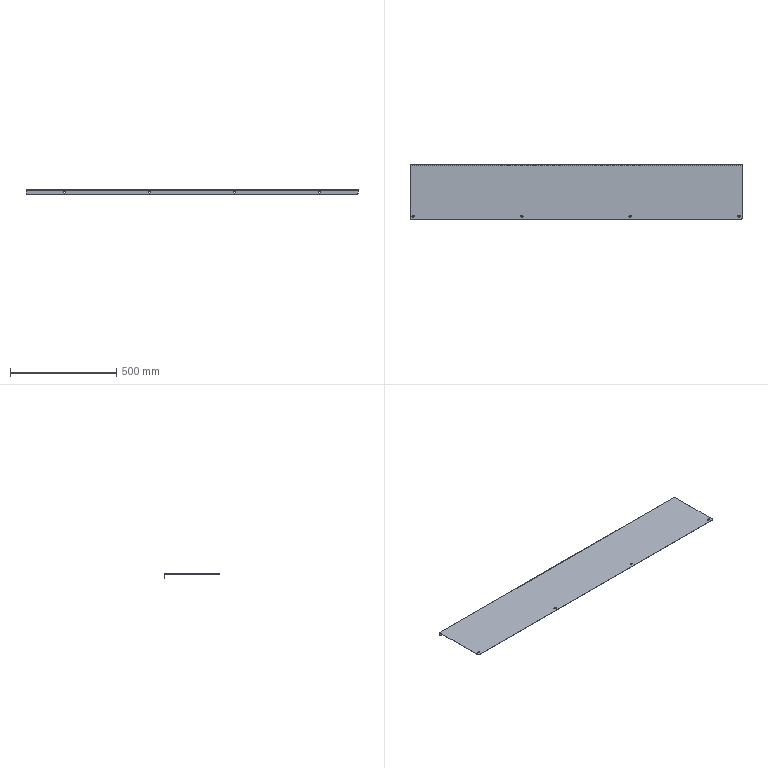Part | SolidWorks | features BaseBody 1 | 1 solid | 62 faces | box 1560 x 258.1 x 20 mm | volume 516469 mm3 | plane 44 | cylinder 18 | commonest cylinder face diameters 7 x12 10 x4 2 x1 4.4 x1